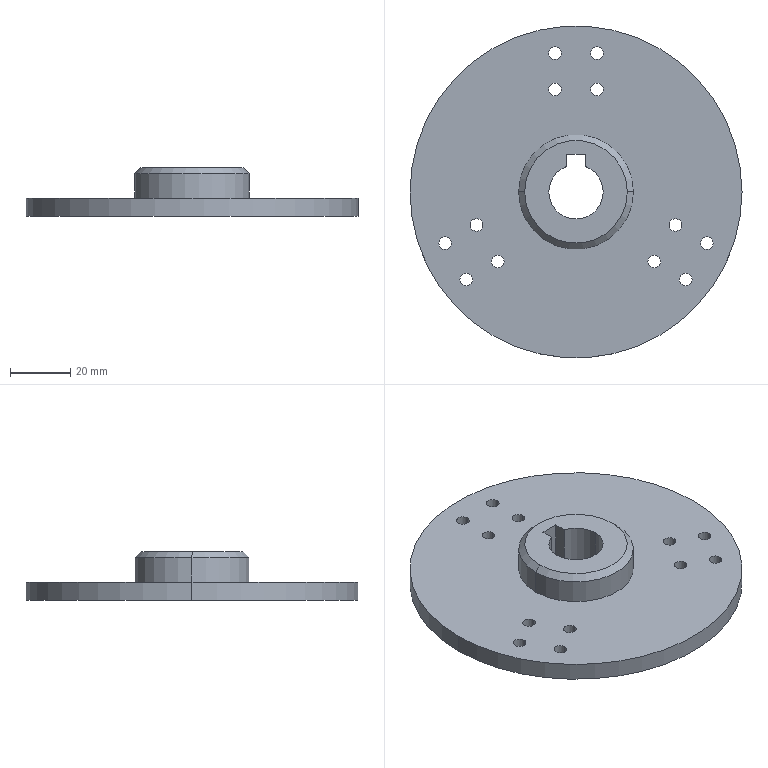Part | STEP file | Cut-off cutter head | 1 solid | 39 faces | box 110 x 110 x 16 mm | volume 62709 mm3 | cylinder 31 | plane 6 | cone 2 | commonest cylinder face diameters 4.2 x24 18 x3 38 x2 110 x2
STEP:
#1=CARTESIAN_POINT('',(17.,0.,16.));
#2=VERTEX_POINT('',#1);
#3=CARTESIAN_POINT('',(-17.,0.,16.));
#4=VERTEX_POINT('',#3);
#5=CARTESIAN_POINT('',(0.,0.,16.));
#6=DIRECTION('',(0.,0.,1.));
#7=DIRECTION('',(1.,0.,0.));
#8=AXIS2_PLACEMENT_3D('',#5,#6,#7);
#9=CIRCLE('',#8,17.);
#10=EDGE_CURVE('',#2,#4,#9,.T.);
#11=ORIENTED_EDGE('',*,*,#10,.F.);
#12=CARTESIAN_POINT('',(19.,0.,14.));
#13=VERTEX_POINT('',#12);
#14=CARTESIAN_POINT('',(17.,0.,16.));
#15=DIRECTION('',(0.7071,0.,-0.7071));
#16=VECTOR('',#15,1000.);
#17=LINE('',#14,#16);
#18=EDGE_CURVE('',#2,#13,#17,.T.);
#19=ORIENTED_EDGE('',*,*,#18,.T.);
#20=CARTESIAN_POINT('',(-19.,0.,14.));
#21=VERTEX_POINT('',#20);
#22=CARTESIAN_POINT('',(0.,0.,14.));
#23=DIRECTION('',(0.,0.,-1.));
#24=DIRECTION('',(1.,0.,0.));
#25=AXIS2_PLACEMENT_3D('',#22,#23,#24);
#26=CIRCLE('',#25,19.);
#27=EDGE_CURVE('',#21,#13,#26,.T.);
#28=ORIENTED_EDGE('',*,*,#27,.F.);
#29=CARTESIAN_POINT('',(-17.,0.,16.));
#30=DIRECTION('',(-0.7071,0.,-0.7071));
#31=VECTOR('',#30,1000.);
#32=LINE('',#29,#31);
#33=EDGE_CURVE('',#4,#21,#32,.T.);
#34=ORIENTED_EDGE('',*,*,#33,.F.);
#35=EDGE_LOOP('',(#11,#19,#28,#34));
#36=FACE_OUTER_BOUND('',#35,.T.);
#37=CARTESIAN_POINT('',(0.,0.,16.));
#38=DIRECTION('',(0.,0.,-1.));
#39=DIRECTION('',(-1.,0.,0.));
#40=AXIS2_PLACEMENT_3D('',#37,#38,#39);
#41=CONICAL_SURFACE('',#40,17.,0.7854);
#42=ADVANCED_FACE('',(#36),#41,.T.);
#43=CARTESIAN_POINT('',(41.237,-16.938,0.));
#44=VERTEX_POINT('',#43);
#45=CARTESIAN_POINT('',(45.437,-16.938,0.));
#46=VERTEX_POINT('',#45);
#47=CARTESIAN_POINT('',(43.337,-16.938,0.));
#48=DIRECTION('',(0.,0.,1.));
#49=DIRECTION('',(1.,0.,0.));
#50=AXIS2_PLACEMENT_3D('',#47,#48,#49);
#51=CIRCLE('',#50,2.1);
#52=EDGE_CURVE('',#44,#46,#51,.T.);
#53=ORIENTED_EDGE('',*,*,#52,.F.);
#54=CARTESIAN_POINT('',(41.237,-16.938,6.));
#55=VERTEX_POINT('',#54);
#56=CARTESIAN_POINT('',(41.237,-16.938,6.));
#57=DIRECTION('',(0.,0.,1.));
#58=VECTOR('',#57,1000.);
#59=LINE('',#56,#58);
#60=EDGE_CURVE('',#44,#55,#59,.T.);
#61=ORIENTED_EDGE('',*,*,#60,.T.);
#62=CARTESIAN_POINT('',(45.437,-16.938,6.));
#63=VERTEX_POINT('',#62);
#64=CARTESIAN_POINT('',(43.337,-16.938,6.));
#65=DIRECTION('',(0.,0.,1.));
#66=DIRECTION('',(1.,0.,0.));
#67=AXIS2_PLACEMENT_3D('',#64,#65,#66);
#68=CIRCLE('',#67,2.1);
#69=EDGE_CURVE('',#55,#63,#68,.T.);
#70=ORIENTED_EDGE('',*,*,#69,.T.);
#71=CARTESIAN_POINT('',(45.437,-16.938,6.));
#72=DIRECTION('',(0.,0.,1.));
#73=VECTOR('',#72,1000.);
#74=LINE('',#71,#73);
#75=EDGE_CURVE('',#46,#63,#74,.T.);
#76=ORIENTED_EDGE('',*,*,#75,.F.);
#77=EDGE_LOOP('',(#53,#61,#70,#76));
#78=FACE_OUTER_BOUND('',#77,.T.);
#79=CARTESIAN_POINT('',(43.337,-16.938,6.));
#80=DIRECTION('',(0.,0.,1.));
#81=DIRECTION('',(1.,0.,0.));
#82=AXIS2_PLACEMENT_3D('',#79,#80,#81);
#83=CYLINDRICAL_SURFACE('',#82,2.1);
#84=ADVANCED_FACE('',(#78),#83,.F.);
#85=CARTESIAN_POINT('',(34.237,-29.062,0.));
#86=VERTEX_POINT('',#85);
#87=CARTESIAN_POINT('',(38.437,-29.062,0.));
#88=VERTEX_POINT('',#87);
#89=CARTESIAN_POINT('',(36.337,-29.062,0.));
#90=DIRECTION('',(0.,0.,1.));
#91=DIRECTION('',(1.,0.,0.));
#92=AXIS2_PLACEMENT_3D('',#89,#90,#91);
#93=CIRCLE('',#92,2.1);
#94=EDGE_CURVE('',#86,#88,#93,.T.);
#95=ORIENTED_EDGE('',*,*,#94,.F.);
#96=CARTESIAN_POINT('',(34.237,-29.062,6.));
#97=VERTEX_POINT('',#96);
#98=CARTESIAN_POINT('',(34.237,-29.062,6.));
#99=DIRECTION('',(0.,0.,1.));
#100=VECTOR('',#99,1000.);
#101=LINE('',#98,#100);
#102=EDGE_CURVE('',#86,#97,#101,.T.);
#103=ORIENTED_EDGE('',*,*,#102,.T.);
#104=CARTESIAN_POINT('',(38.437,-29.062,6.));
#105=VERTEX_POINT('',#104);
#106=CARTESIAN_POINT('',(36.337,-29.062,6.));
#107=DIRECTION('',(0.,0.,1.));
#108=DIRECTION('',(1.,0.,0.));
#109=AXIS2_PLACEMENT_3D('',#106,#107,#108);
#110=CIRCLE('',#109,2.1);
#111=EDGE_CURVE('',#97,#105,#110,.T.);
#112=ORIENTED_EDGE('',*,*,#111,.T.);
#113=CARTESIAN_POINT('',(38.437,-29.062,6.));
#114=DIRECTION('',(0.,0.,1.));
#115=VECTOR('',#114,1000.);
#116=LINE('',#113,#115);
#117=EDGE_CURVE('',#88,#105,#116,.T.);
#118=ORIENTED_EDGE('',*,*,#117,.F.);
#119=EDGE_LOOP('',(#95,#103,#112,#118));
#120=FACE_OUTER_BOUND('',#119,.T.);
#121=CARTESIAN_POINT('',(36.337,-29.062,6.));
#122=DIRECTION('',(0.,0.,1.));
#123=DIRECTION('',(1.,0.,0.));
#124=AXIS2_PLACEMENT_3D('',#121,#122,#123);
#125=CYLINDRICAL_SURFACE('',#124,2.1);
#126=ADVANCED_FACE('',(#120),#125,.F.);
#127=CARTESIAN_POINT('',(23.845,-23.062,0.));
#128=VERTEX_POINT('',#127);
#129=CARTESIAN_POINT('',(28.045,-23.062,0.));
#130=VERTEX_POINT('',#129);
#131=CARTESIAN_POINT('',(25.945,-23.062,0.));
#132=DIRECTION('',(0.,0.,1.));
#133=DIRECTION('',(1.,0.,0.));
#134=AXIS2_PLACEMENT_3D('',#131,#132,#133);
#135=CIRCLE('',#134,2.1);
#136=EDGE_CURVE('',#128,#130,#135,.T.);
#137=ORIENTED_EDGE('',*,*,#136,.F.);
#138=CARTESIAN_POINT('',(23.845,-23.062,6.));
#139=VERTEX_POINT('',#138);
#140=CARTESIAN_POINT('',(23.845,-23.062,6.));
#141=DIRECTION('',(0.,0.,1.));
#142=VECTOR('',#141,1000.);
#143=LINE('',#140,#142);
#144=EDGE_CURVE('',#128,#139,#143,.T.);
#145=ORIENTED_EDGE('',*,*,#144,.T.);
#146=CARTESIAN_POINT('',(28.045,-23.062,6.));
#147=VERTEX_POINT('',#146);
#148=CARTESIAN_POINT('',(25.945,-23.062,6.));
#149=DIRECTION('',(0.,0.,1.));
#150=DIRECTION('',(1.,0.,0.));
#151=AXIS2_PLACEMENT_3D('',#148,#149,#150);
#152=CIRCLE('',#151,2.1);
#153=EDGE_CURVE('',#139,#147,#152,.T.);
#154=ORIENTED_EDGE('',*,*,#153,.T.);
#155=CARTESIAN_POINT('',(28.045,-23.062,6.));
#156=DIRECTION('',(0.,0.,1.));
#157=VECTOR('',#156,1000.);
#158=LINE('',#155,#157);
#159=EDGE_CURVE('',#130,#147,#158,.T.);
#160=ORIENTED_EDGE('',*,*,#159,.F.);
#161=EDGE_LOOP('',(#137,#145,#154,#160));
#162=FACE_OUTER_BOUND('',#161,.T.);
#163=CARTESIAN_POINT('',(25.945,-23.062,6.));
#164=DIRECTION('',(0.,0.,1.));
#165=DIRECTION('',(1.,0.,0.));
#166=AXIS2_PLACEMENT_3D('',#163,#164,#165);
#167=CYLINDRICAL_SURFACE('',#166,2.1);
#168=ADVANCED_FACE('',(#162),#167,.F.);
#169=CARTESIAN_POINT('',(30.845,-10.938,0.));
#170=VERTEX_POINT('',#169);
#171=CARTESIAN_POINT('',(35.045,-10.938,0.));
#172=VERTEX_POINT('',#171);
#173=CARTESIAN_POINT('',(32.945,-10.938,0.));
#174=DIRECTION('',(0.,0.,1.));
#175=DIRECTION('',(1.,0.,0.));
#176=AXIS2_PLACEMENT_3D('',#173,#174,#175);
#177=CIRCLE('',#176,2.1);
#178=EDGE_CURVE('',#170,#172,#177,.T.);
#179=ORIENTED_EDGE('',*,*,#178,.F.);
#180=CARTESIAN_POINT('',(30.845,-10.938,6.));
#181=VERTEX_POINT('',#180);
#182=CARTESIAN_POINT('',(30.845,-10.938,6.));
#183=DIRECTION('',(0.,0.,1.));
#184=VECTOR('',#183,1000.);
#185=LINE('',#182,#184);
#186=EDGE_CURVE('',#170,#181,#185,.T.);
#187=ORIENTED_EDGE('',*,*,#186,.T.);
#188=CARTESIAN_POINT('',(35.045,-10.938,6.));
#189=VERTEX_POINT('',#188);
#190=CARTESIAN_POINT('',(32.945,-10.938,6.));
#191=DIRECTION('',(0.,0.,1.));
#192=DIRECTION('',(1.,0.,0.));
#193=AXIS2_PLACEMENT_3D('',#190,#191,#192);
#194=CIRCLE('',#193,2.1);
#195=EDGE_CURVE('',#181,#189,#194,.T.);
#196=ORIENTED_EDGE('',*,*,#195,.T.);
#197=CARTESIAN_POINT('',(35.045,-10.938,6.));
#198=DIRECTION('',(0.,0.,1.));
#199=VECTOR('',#198,1000.);
#200=LINE('',#197,#199);
#201=EDGE_CURVE('',#172,#189,#200,.T.);
#202=ORIENTED_EDGE('',*,*,#201,.F.);
#203=EDGE_LOOP('',(#179,#187,#196,#202));
#204=FACE_OUTER_BOUND('',#203,.T.);
#205=CARTESIAN_POINT('',(32.945,-10.938,6.));
#206=DIRECTION('',(0.,0.,1.));
#207=DIRECTION('',(1.,0.,0.));
#208=AXIS2_PLACEMENT_3D('',#205,#206,#207);
#209=CYLINDRICAL_SURFACE('',#208,2.1);
#210=ADVANCED_FACE('',(#204),#209,.F.);
#211=CARTESIAN_POINT('',(-38.437,-29.062,0.));
#212=VERTEX_POINT('',#211);
#213=CARTESIAN_POINT('',(-34.237,-29.062,0.));
#214=VERTEX_POINT('',#213);
#215=CARTESIAN_POINT('',(-36.337,-29.062,0.));
#216=DIRECTION('',(0.,0.,1.));
#217=DIRECTION('',(1.,0.,0.));
#218=AXIS2_PLACEMENT_3D('',#215,#216,#217);
#219=CIRCLE('',#218,2.1);
#220=EDGE_CURVE('',#212,#214,#219,.T.);
#221=ORIENTED_EDGE('',*,*,#220,.F.);
#222=CARTESIAN_POINT('',(-38.437,-29.062,6.));
#223=VERTEX_POINT('',#222);
#224=CARTESIAN_POINT('',(-38.437,-29.062,6.));
#225=DIRECTION('',(0.,0.,1.));
#226=VECTOR('',#225,1000.);
#227=LINE('',#224,#226);
#228=EDGE_CURVE('',#212,#223,#227,.T.);
#229=ORIENTED_EDGE('',*,*,#228,.T.);
#230=CARTESIAN_POINT('',(-34.237,-29.062,6.));
#231=VERTEX_POINT('',#230);
#232=CARTESIAN_POINT('',(-36.337,-29.062,6.));
#233=DIRECTION('',(0.,0.,1.));
#234=DIRECTION('',(1.,0.,0.));
#235=AXIS2_PLACEMENT_3D('',#232,#233,#234);
#236=CIRCLE('',#235,2.1);
#237=EDGE_CURVE('',#223,#231,#236,.T.);
#238=ORIENTED_EDGE('',*,*,#237,.T.);
#239=CARTESIAN_POINT('',(-34.237,-29.062,6.));
#240=DIRECTION('',(0.,0.,1.));
#241=VECTOR('',#240,1000.);
#242=LINE('',#239,#241);
#243=EDGE_CURVE('',#214,#231,#242,.T.);
#244=ORIENTED_EDGE('',*,*,#243,.F.);
#245=EDGE_LOOP('',(#221,#229,#238,#244));
#246=FACE_OUTER_BOUND('',#245,.T.);
#247=CARTESIAN_POINT('',(-36.337,-29.062,6.));
#248=DIRECTION('',(0.,0.,1.));
#249=DIRECTION('',(1.,0.,0.));
#250=AXIS2_PLACEMENT_3D('',#247,#248,#249);
#251=CYLINDRICAL_SURFACE('',#250,2.1);
#252=ADVANCED_FACE('',(#246),#251,.F.);
#253=CARTESIAN_POINT('',(-45.437,-16.938,0.));
#254=VERTEX_POINT('',#253);
#255=CARTESIAN_POINT('',(-41.237,-16.938,0.));
#256=VERTEX_POINT('',#255);
#257=CARTESIAN_POINT('',(-43.337,-16.938,0.));
#258=DIRECTION('',(0.,0.,1.));
#259=DIRECTION('',(1.,0.,0.));
#260=AXIS2_PLACEMENT_3D('',#257,#258,#259);
#261=CIRCLE('',#260,2.1);
#262=EDGE_CURVE('',#254,#256,#261,.T.);
#263=ORIENTED_EDGE('',*,*,#262,.F.);
#264=CARTESIAN_POINT('',(-45.437,-16.938,6.));
#265=VERTEX_POINT('',#264);
#266=CARTESIAN_POINT('',(-45.437,-16.938,6.));
#267=DIRECTION('',(0.,0.,1.));
#268=VECTOR('',#267,1000.);
#269=LINE('',#266,#268);
#270=EDGE_CURVE('',#254,#265,#269,.T.);
#271=ORIENTED_EDGE('',*,*,#270,.T.);
#272=CARTESIAN_POINT('',(-41.237,-16.938,6.));
#273=VERTEX_POINT('',#272);
#274=CARTESIAN_POINT('',(-43.337,-16.938,6.));
#275=DIRECTION('',(0.,0.,1.));
#276=DIRECTION('',(1.,0.,0.));
#277=AXIS2_PLACEMENT_3D('',#274,#275,#276);
#278=CIRCLE('',#277,2.1);
#279=EDGE_CURVE('',#265,#273,#278,.T.);
#280=ORIENTED_EDGE('',*,*,#279,.T.);
#281=CARTESIAN_POINT('',(-41.237,-16.938,6.));
#282=DIRECTION('',(0.,0.,1.));
#283=VECTOR('',#282,1000.);
#284=LINE('',#281,#283);
#285=EDGE_CURVE('',#256,#273,#284,.T.);
#286=ORIENTED_EDGE('',*,*,#285,.F.);
#287=EDGE_LOOP('',(#263,#271,#280,#286));
#288=FACE_OUTER_BOUND('',#287,.T.);
#289=CARTESIAN_POINT('',(-43.337,-16.938,6.));
#290=DIRECTION('',(0.,0.,1.));
#291=DIRECTION('',(1.,0.,0.));
#292=AXIS2_PLACEMENT_3D('',#289,#290,#291);
#293=CYLINDRICAL_SURFACE('',#292,2.1);
#294=ADVANCED_FACE('',(#288),#293,.F.);
#295=CARTESIAN_POINT('',(-35.045,-10.938,0.));
#296=VERTEX_POINT('',#295);
#297=CARTESIAN_POINT('',(-30.845,-10.938,0.));
#298=VERTEX_POINT('',#297);
#299=CARTESIAN_POINT('',(-32.945,-10.938,0.));
#300=DIRECTION('',(0.,0.,1.));
#301=DIRECTION('',(1.,0.,0.));
#302=AXIS2_PLACEMENT_3D('',#299,#300,#301);
#303=CIRCLE('',#302,2.1);
#304=EDGE_CURVE('',#296,#298,#303,.T.);
#305=ORIENTED_EDGE('',*,*,#304,.F.);
#306=CARTESIAN_POINT('',(-35.045,-10.938,6.));
#307=VERTEX_POINT('',#306);
#308=CARTESIAN_POINT('',(-35.045,-10.938,6.));
#309=DIRECTION('',(0.,0.,1.));
#310=VECTOR('',#309,1000.);
#311=LINE('',#308,#310);
#312=EDGE_CURVE('',#296,#307,#311,.T.);
#313=ORIENTED_EDGE('',*,*,#312,.T.);
#314=CARTESIAN_POINT('',(-30.845,-10.938,6.));
#315=VERTEX_POINT('',#314);
#316=CARTESIAN_POINT('',(-32.945,-10.938,6.));
#317=DIRECTION('',(0.,0.,1.));
#318=DIRECTION('',(1.,0.,0.));
#319=AXIS2_PLACEMENT_3D('',#316,#317,#318);
#320=CIRCLE('',#319,2.1);
#321=EDGE_CURVE('',#307,#315,#320,.T.);
#322=ORIENTED_EDGE('',*,*,#321,.T.);
#323=CARTESIAN_POINT('',(-30.845,-10.938,6.));
#324=DIRECTION('',(0.,0.,1.));
#325=VECTOR('',#324,1000.);
#326=LINE('',#323,#325);
#327=EDGE_CURVE('',#298,#315,#326,.T.);
#328=ORIENTED_EDGE('',*,*,#327,.F.);
#329=EDGE_LOOP('',(#305,#313,#322,#328));
#330=FACE_OUTER_BOUND('',#329,.T.);
#331=CARTESIAN_POINT('',(-32.945,-10.938,6.));
#332=DIRECTION('',(0.,0.,1.));
#333=DIRECTION('',(1.,0.,0.));
#334=AXIS2_PLACEMENT_3D('',#331,#332,#333);
#335=CYLINDRICAL_SURFACE('',#334,2.1);
#336=ADVANCED_FACE('',(#330),#335,.F.);
#337=CARTESIAN_POINT('',(-28.045,-23.062,0.));
#338=VERTEX_POINT('',#337);
#339=CARTESIAN_POINT('',(-23.845,-23.062,0.));
#340=VERTEX_POINT('',#339);
#341=CARTESIAN_POINT('',(-25.945,-23.062,0.));
#342=DIRECTION('',(0.,0.,1.));
#343=DIRECTION('',(1.,0.,0.));
#344=AXIS2_PLACEMENT_3D('',#341,#342,#343);
#345=CIRCLE('',#344,2.1);
#346=EDGE_CURVE('',#338,#340,#345,.T.);
#347=ORIENTED_EDGE('',*,*,#346,.F.);
#348=CARTESIAN_POINT('',(-28.045,-23.062,6.));
#349=VERTEX_POINT('',#348);
#350=CARTESIAN_POINT('',(-28.045,-23.062,6.));
#351=DIRECTION('',(0.,0.,1.));
#352=VECTOR('',#351,1000.);
#353=LINE('',#350,#352);
#354=EDGE_CURVE('',#338,#349,#353,.T.);
#355=ORIENTED_EDGE('',*,*,#354,.T.);
#356=CARTESIAN_POINT('',(-23.845,-23.062,6.));
#357=VERTEX_POINT('',#356);
#358=CARTESIAN_POINT('',(-25.945,-23.062,6.));
#359=DIRECTION('',(0.,0.,1.));
#360=DIRECTION('',(1.,0.,0.));
#361=AXIS2_PLACEMENT_3D('',#358,#359,#360);
#362=CIRCLE('',#361,2.1);
#363=EDGE_CURVE('',#349,#357,#362,.T.);
#364=ORIENTED_EDGE('',*,*,#363,.T.);
#365=CARTESIAN_POINT('',(-23.845,-23.062,6.));
#366=DIRECTION('',(0.,0.,1.));
#367=VECTOR('',#366,1000.);
#368=LINE('',#365,#367);
#369=EDGE_CURVE('',#340,#357,#368,.T.);
#370=ORIENTED_EDGE('',*,*,#369,.F.);
#371=EDGE_LOOP('',(#347,#355,#364,#370));
#372=FACE_OUTER_BOUND('',#371,.T.);
#373=CARTESIAN_POINT('',(-25.945,-23.062,6.));
#374=DIRECTION('',(0.,0.,1.));
#375=DIRECTION('',(1.,0.,0.));
#376=AXIS2_PLACEMENT_3D('',#373,#374,#375);
#377=CYLINDRICAL_SURFACE('',#376,2.1);
#378=ADVANCED_FACE('',(#372),#377,.F.);
#379=CARTESIAN_POINT('',(-9.1,46.,0.));
#380=VERTEX_POINT('',#379);
#381=CARTESIAN_POINT('',(-4.9,46.,0.));
#382=VERTEX_POINT('',#381);
#383=CARTESIAN_POINT('',(-7.,46.,0.));
#384=DIRECTION('',(0.,0.,1.));
#385=DIRECTION('',(1.,0.,0.));
#386=AXIS2_PLACEMENT_3D('',#383,#384,#385);
#387=CIRCLE('',#386,2.1);
#388=EDGE_CURVE('',#380,#382,#387,.T.);
#389=ORIENTED_EDGE('',*,*,#388,.F.);
#390=CARTESIAN_POINT('',(-9.1,46.,6.));
#391=VERTEX_POINT('',#390);
#392=CARTESIAN_POINT('',(-9.1,46.,6.));
#393=DIRECTION('',(0.,0.,1.));
#394=VECTOR('',#393,1000.);
#395=LINE('',#392,#394);
#396=EDGE_CURVE('',#380,#391,#395,.T.);
#397=ORIENTED_EDGE('',*,*,#396,.T.);
#398=CARTESIAN_POINT('',(-4.9,46.,6.));
#399=VERTEX_POINT('',#398);
#400=CARTESIAN_POINT('',(-7.,46.,6.));
#401=DIRECTION('',(0.,0.,1.));
#402=DIRECTION('',(1.,0.,0.));
#403=AXIS2_PLACEMENT_3D('',#400,#401,#402);
#404=CIRCLE('',#403,2.1);
#405=EDGE_CURVE('',#391,#399,#404,.T.);
#406=ORIENTED_EDGE('',*,*,#405,.T.);
#407=CARTESIAN_POINT('',(-4.9,46.,6.));
#408=DIRECTION('',(0.,0.,1.));
#409=VECTOR('',#408,1000.);
#410=LINE('',#407,#409);
#411=EDGE_CURVE('',#382,#399,#410,.T.);
#412=ORIENTED_EDGE('',*,*,#411,.F.);
#413=EDGE_LOOP('',(#389,#397,#406,#412));
#414=FACE_OUTER_BOUND('',#413,.T.);
#415=CARTESIAN_POINT('',(-7.,46.,6.));
#416=DIRECTION('',(0.,0.,1.));
#417=DIRECTION('',(1.,0.,0.));
#418=AXIS2_PLACEMENT_3D('',#415,#416,#417);
#419=CYLINDRICAL_SURFACE('',#418,2.1);
#420=ADVANCED_FACE('',(#414),#419,.F.);
#421=CARTESIAN_POINT('',(4.9,46.,0.));
#422=VERTEX_POINT('',#421);
#423=CARTESIAN_POINT('',(9.1,46.,0.));
#424=VERTEX_POINT('',#423);
#425=CARTESIAN_POINT('',(7.,46.,0.));
#426=DIRECTION('',(0.,0.,1.));
#427=DIRECTION('',(1.,0.,0.));
#428=AXIS2_PLACEMENT_3D('',#425,#426,#427);
#429=CIRCLE('',#428,2.1);
#430=EDGE_CURVE('',#422,#424,#429,.T.);
#431=ORIENTED_EDGE('',*,*,#430,.F.);
#432=CARTESIAN_POINT('',(4.9,46.,6.));
#433=VERTEX_POINT('',#432);
#434=CARTESIAN_POINT('',(4.9,46.,6.));
#435=DIRECTION('',(0.,0.,1.));
#436=VECTOR('',#435,1000.);
#437=LINE('',#434,#436);
#438=EDGE_CURVE('',#422,#433,#437,.T.);
#439=ORIENTED_EDGE('',*,*,#438,.T.);
#440=CARTESIAN_POINT('',(9.1,46.,6.));
#441=VERTEX_POINT('',#440);
#442=CARTESIAN_POINT('',(7.,46.,6.));
#443=DIRECTION('',(0.,0.,1.));
#444=DIRECTION('',(1.,0.,0.));
#445=AXIS2_PLACEMENT_3D('',#442,#443,#444);
#446=CIRCLE('',#445,2.1);
#447=EDGE_CURVE('',#433,#441,#446,.T.);
#448=ORIENTED_EDGE('',*,*,#447,.T.);
#449=CARTESIAN_POINT('',(9.1,46.,6.));
#450=DIRECTION('',(0.,0.,1.));
#451=VECTOR('',#450,1000.);
#452=LINE('',#449,#451);
#453=EDGE_CURVE('',#424,#441,#452,.T.);
#454=ORIENTED_EDGE('',*,*,#453,.F.);
#455=EDGE_LOOP('',(#431,#439,#448,#454));
#456=FACE_OUTER_BOUND('',#455,.T.);
#457=CARTESIAN_POINT('',(7.,46.,6.));
#458=DIRECTION('',(0.,0.,1.));
#459=DIRECTION('',(1.,0.,0.));
#460=AXIS2_PLACEMENT_3D('',#457,#458,#459);
#461=CYLINDRICAL_SURFACE('',#460,2.1);
#462=ADVANCED_FACE('',(#456),#461,.F.);
#463=CARTESIAN_POINT('',(4.9,34.,0.));
#464=VERTEX_POINT('',#463);
#465=CARTESIAN_POINT('',(9.1,34.,0.));
#466=VERTEX_POINT('',#465);
#467=CARTESIAN_POINT('',(7.,34.,0.));
#468=DIRECTION('',(0.,0.,1.));
#469=DIRECTION('',(1.,0.,0.));
#470=AXIS2_PLACEMENT_3D('',#467,#468,#469);
#471=CIRCLE('',#470,2.1);
#472=EDGE_CURVE('',#464,#466,#471,.T.);
#473=ORIENTED_EDGE('',*,*,#472,.F.);
#474=CARTESIAN_POINT('',(4.9,34.,6.));
#475=VERTEX_POINT('',#474);
#476=CARTESIAN_POINT('',(4.9,34.,6.));
#477=DIRECTION('',(0.,0.,1.));
#478=VECTOR('',#477,1000.);
#479=LINE('',#476,#478);
#480=EDGE_CURVE('',#464,#475,#479,.T.);
#481=ORIENTED_EDGE('',*,*,#480,.T.);
#482=CARTESIAN_POINT('',(9.1,34.,6.));
#483=VERTEX_POINT('',#482);
#484=CARTESIAN_POINT('',(7.,34.,6.));
#485=DIRECTION('',(0.,0.,1.));
#486=DIRECTION('',(1.,0.,0.));
#487=AXIS2_PLACEMENT_3D('',#484,#485,#486);
#488=CIRCLE('',#487,2.1);
#489=EDGE_CURVE('',#475,#483,#488,.T.);
#490=ORIENTED_EDGE('',*,*,#489,.T.);
#491=CARTESIAN_POINT('',(9.1,34.,6.));
#492=DIRECTION('',(0.,0.,1.));
#493=VECTOR('',#492,1000.);
#494=LINE('',#491,#493);
#495=EDGE_CURVE('',#466,#483,#494,.T.);
#496=ORIENTED_EDGE('',*,*,#495,.F.);
#497=EDGE_LOOP('',(#473,#481,#490,#496));
#498=FACE_OUTER_BOUND('',#497,.T.);
#499=CARTESIAN_POINT('',(7.,34.,6.));
#500=DIRECTION('',(0.,0.,1.));
#501=DIRECTION('',(1.,0.,0.));
#502=AXIS2_PLACEMENT_3D('',#499,#500,#501);
#503=CYLINDRICAL_SURFACE('',#502,2.1);
#504=ADVANCED_FACE('',(#498),#503,.F.);
#505=CARTESIAN_POINT('',(-9.1,34.,0.));
#506=VERTEX_POINT('',#505);
#507=CARTESIAN_POINT('',(-4.9,34.,0.));
#508=VERTEX_POINT('',#507);
#509=CARTESIAN_POINT('',(-7.,34.,0.));
#510=DIRECTION('',(0.,0.,1.));
#511=DIRECTION('',(1.,0.,0.));
#512=AXIS2_PLACEMENT_3D('',#509,#510,#511);
#513=CIRCLE('',#512,2.1);
#514=EDGE_CURVE('',#506,#508,#513,.T.);
#515=ORIENTED_EDGE('',*,*,#514,.F.);
#516=CARTESIAN_POINT('',(-9.1,34.,6.));
#517=VERTEX_POINT('',#516);
#518=CARTESIAN_POINT('',(-9.1,34.,6.));
#519=DIRECTION('',(0.,0.,1.));
#520=VECTOR('',#519,1000.);
#521=LINE('',#518,#520);
#522=EDGE_CURVE('',#506,#517,#521,.T.);
#523=ORIENTED_EDGE('',*,*,#522,.T.);
#524=CARTESIAN_POINT('',(-4.9,34.,6.));
#525=VERTEX_POINT('',#524);
#526=CARTESIAN_POINT('',(-7.,34.,6.));
#527=DIRECTION('',(0.,0.,1.));
#528=DIRECTION('',(1.,0.,0.));
#529=AXIS2_PLACEMENT_3D('',#526,#527,#528);
#530=CIRCLE('',#529,2.1);
#531=EDGE_CURVE('',#517,#525,#530,.T.);
#532=ORIENTED_EDGE('',*,*,#531,.T.);
#533=CARTESIAN_POINT('',(-4.9,34.,6.));
#534=DIRECTION('',(0.,0.,1.));
#535=VECTOR('',#534,1000.);
#536=LINE('',#533,#535);
#537=EDGE_CURVE('',#508,#525,#536,.T.);
#538=ORIENTED_EDGE('',*,*,#537,.F.);
#539=EDGE_LOOP('',(#515,#523,#532,#538));
#540=FACE_OUTER_BOUND('',#539,.T.);
#541=CARTESIAN_POINT('',(-7.,34.,6.));
#542=DIRECTION('',(0.,0.,1.));
#543=DIRECTION('',(1.,0.,0.));
#544=AXIS2_PLACEMENT_3D('',#541,#542,#543);
#545=CYLINDRICAL_SURFACE('',#544,2.1);
#546=ADVANCED_FACE('',(#540),#545,.F.);
#547=CARTESIAN_POINT('',(-9.,0.,16.));
#548=VERTEX_POINT('',#547);
#549=CARTESIAN_POINT('',(9.,0.,16.));
#550=VERTEX_POINT('',#549);
#551=CARTESIAN_POINT('',(0.,0.,16.));
#552=DIRECTION('',(0.,0.,1.));
#553=DIRECTION('',(1.,0.,0.));
#554=AXIS2_PLACEMENT_3D('',#551,#552,#553);
#555=CIRCLE('',#554,9.);
#556=EDGE_CURVE('',#548,#550,#555,.T.);
#557=ORIENTED_EDGE('',*,*,#556,.T.);
#558=CARTESIAN_POINT('',(9.,0.,0.));
#559=VERTEX_POINT('',#558);
#560=CARTESIAN_POINT('',(9.,0.,16.));
#561=DIRECTION('',(0.,0.,-1.));
#562=VECTOR('',#561,1000.);
#563=LINE('',#560,#562);
#564=EDGE_CURVE('',#550,#559,#563,.T.);
#565=ORIENTED_EDGE('',*,*,#564,.T.);
#566=CARTESIAN_POINT('',(-9.,0.,0.));
#567=VERTEX_POINT('',#566);
#568=CARTESIAN_POINT('',(0.,0.,0.));
#569=DIRECTION('',(0.,0.,1.));
#570=DIRECTION('',(1.,0.,0.));
#571=AXIS2_PLACEMENT_3D('',#568,#569,#570);
#572=CIRCLE('',#571,9.);
#573=EDGE_CURVE('',#567,#559,#572,.T.);
#574=ORIENTED_EDGE('',*,*,#573,.F.);
#575=CARTESIAN_POINT('',(-9.,0.,16.));
#576=DIRECTION('',(0.,0.,-1.));
#577=VECTOR('',#576,1000.);
#578=LINE('',#575,#577);
#579=EDGE_CURVE('',#548,#567,#578,.T.);
#580=ORIENTED_EDGE('',*,*,#579,.F.);
#581=EDGE_LOOP('',(#557,#565,#574,#580));
#582=FACE_OUTER_BOUND('',#581,.T.);
#583=CARTESIAN_POINT('',(0.,0.,16.));
#584=DIRECTION('',(0.,0.,-1.));
#585=DIRECTION('',(-1.,0.,0.));
#586=AXIS2_PLACEMENT_3D('',#583,#584,#585);
#587=CYLINDRICAL_SURFACE('',#586,9.);
#588=ADVANCED_FACE('',(#582),#587,.F.);
#589=CARTESIAN_POINT('',(-3.,8.485,16.));
#590=VERTEX_POINT('',#589);
#591=CARTESIAN_POINT('',(0.,0.,16.));
#592=DIRECTION('',(0.,0.,1.));
#593=DIRECTION('',(1.,0.,0.));
#594=AXIS2_PLACEMENT_3D('',#591,#592,#593);
#595=CIRCLE('',#594,9.);
#596=EDGE_CURVE('',#590,#548,#595,.T.);
#597=ORIENTED_EDGE('',*,*,#596,.T.);
#598=ORIENTED_EDGE('',*,*,#579,.T.);
#599=CARTESIAN_POINT('',(-3.,8.485,0.));
#600=VERTEX_POINT('',#599);
#601=CARTESIAN_POINT('',(0.,0.,0.));
#602=DIRECTION('',(0.,0.,1.));
#603=DIRECTION('',(1.,0.,0.));
#604=AXIS2_PLACEMENT_3D('',#601,#602,#603);
#605=CIRCLE('',#604,9.);
#606=EDGE_CURVE('',#600,#567,#605,.T.);
#607=ORIENTED_EDGE('',*,*,#606,.F.);
#608=CARTESIAN_POINT('',(-3.,8.485,16.));
#609=DIRECTION('',(0.,0.,-1.));
#610=VECTOR('',#609,1000.);
#611=LINE('',#608,#610);
#612=EDGE_CURVE('',#590,#600,#611,.T.);
#613=ORIENTED_EDGE('',*,*,#612,.F.);
#614=EDGE_LOOP('',(#597,#598,#607,#613));
#615=FACE_OUTER_BOUND('',#614,.T.);
#616=CARTESIAN_POINT('',(0.,0.,16.));
#617=DIRECTION('',(0.,0.,-1.));
#618=DIRECTION('',(-1.,0.,0.));
#619=AXIS2_PLACEMENT_3D('',#616,#617,#618);
#620=CYLINDRICAL_SURFACE('',#619,9.);
#621=ADVANCED_FACE('',(#615),#620,.F.);
#622=ORIENTED_EDGE('',*,*,#27,.T.);
#623=CARTESIAN_POINT('',(19.,0.,6.));
#624=VERTEX_POINT('',#623);
#625=CARTESIAN_POINT('',(19.,0.,16.));
#626=DIRECTION('',(0.,0.,-1.));
#627=VECTOR('',#626,1000.);
#628=LINE('',#625,#627);
#629=EDGE_CURVE('',#13,#624,#628,.T.);
#630=ORIENTED_EDGE('',*,*,#629,.T.);
#631=CARTESIAN_POINT('',(-19.,0.,6.));
#632=VERTEX_POINT('',#631);
#633=CARTESIAN_POINT('',(0.,0.,6.));
#634=DIRECTION('',(0.,0.,1.));
#635=DIRECTION('',(1.,0.,0.));
#636=AXIS2_PLACEMENT_3D('',#633,#634,#635);
#637=CIRCLE('',#636,19.);
#638=EDGE_CURVE('',#624,#632,#637,.T.);
#639=ORIENTED_EDGE('',*,*,#638,.T.);
#640=CARTESIAN_POINT('',(-19.,0.,16.));
#641=DIRECTION('',(0.,0.,-1.));
#642=VECTOR('',#641,1000.);
#643=LINE('',#640,#642);
#644=EDGE_CURVE('',#21,#632,#643,.T.);
#645=ORIENTED_EDGE('',*,*,#644,.F.);
#646=EDGE_LOOP('',(#622,#630,#639,#645));
#647=FACE_OUTER_BOUND('',#646,.T.);
#648=CARTESIAN_POINT('',(0.,0.,16.));
#649=DIRECTION('',(0.,0.,-1.));
#650=DIRECTION('',(-1.,0.,0.));
#651=AXIS2_PLACEMENT_3D('',#648,#649,#650);
#652=CYLINDRICAL_SURFACE('',#651,19.);
#653=ADVANCED_FACE('',(#647),#652,.T.);
#654=CARTESIAN_POINT('',(55.,0.,6.));
#655=VERTEX_POINT('',#654);
#656=CARTESIAN_POINT('',(-55.,0.,6.));
#657=VERTEX_POINT('',#656);
#658=CARTESIAN_POINT('',(0.,0.,6.));
#659=DIRECTION('',(0.,0.,1.));
#660=DIRECTION('',(1.,0.,0.));
#661=AXIS2_PLACEMENT_3D('',#658,#659,#660);
#662=CIRCLE('',#661,55.);
#663=EDGE_CURVE('',#655,#657,#662,.T.);
#664=ORIENTED_EDGE('',*,*,#663,.F.);
#665=CARTESIAN_POINT('',(55.,0.,0.));
#666=VERTEX_POINT('',#665);
#667=CARTESIAN_POINT('',(55.,0.,6.));
#668=DIRECTION('',(0.,0.,-1.));
#669=VECTOR('',#668,1000.);
#670=LINE('',#667,#669);
#671=EDGE_CURVE('',#655,#666,#670,.T.);
#672=ORIENTED_EDGE('',*,*,#671,.T.);
#673=CARTESIAN_POINT('',(-55.,0.,0.));
#674=VERTEX_POINT('',#673);
#675=CARTESIAN_POINT('',(0.,0.,0.));
#676=DIRECTION('',(0.,0.,1.));
#677=DIRECTION('',(1.,0.,0.));
#678=AXIS2_PLACEMENT_3D('',#675,#676,#677);
#679=CIRCLE('',#678,55.);
#680=EDGE_CURVE('',#666,#674,#679,.T.);
#681=ORIENTED_EDGE('',*,*,#680,.T.);
#682=CARTESIAN_POINT('',(-55.,0.,6.));
#683=DIRECTION('',(0.,0.,-1.));
#684=VECTOR('',#683,1000.);
#685=LINE('',#682,#684);
#686=EDGE_CURVE('',#657,#674,#685,.T.);
#687=ORIENTED_EDGE('',*,*,#686,.F.);
#688=EDGE_LOOP('',(#664,#672,#681,#687));
#689=FACE_OUTER_BOUND('',#688,.T.);
#690=CARTESIAN_POINT('',(0.,0.,6.));
#691=DIRECTION('',(0.,0.,-1.));
#692=DIRECTION('',(-1.,0.,0.));
#693=AXIS2_PLACEMENT_3D('',#690,#691,#692);
#694=CYLINDRICAL_SURFACE('',#693,55.);
#695=ADVANCED_FACE('',(#689),#694,.T.);
#696=ORIENTED_EDGE('',*,*,#671,.F.);
#697=CARTESIAN_POINT('',(0.,0.,6.));
#698=DIRECTION('',(0.,0.,1.));
#699=DIRECTION('',(1.,0.,0.));
#700=AXIS2_PLACEMENT_3D('',#697,#698,#699);
#701=CIRCLE('',#700,55.);
#702=EDGE_CURVE('',#657,#655,#701,.T.);
#703=ORIENTED_EDGE('',*,*,#702,.F.);
#704=ORIENTED_EDGE('',*,*,#686,.T.);
#705=CARTESIAN_POINT('',(0.,0.,0.));
#706=DIRECTION('',(0.,0.,1.));
#707=DIRECTION('',(1.,0.,0.));
#708=AXIS2_PLACEMENT_3D('',#705,#706,#707);
#709=CIRCLE('',#708,55.);
#710=EDGE_CURVE('',#674,#666,#709,.T.);
#711=ORIENTED_EDGE('',*,*,#710,.T.);
#712=EDGE_LOOP('',(#696,#703,#704,#711));
#713=FACE_OUTER_BOUND('',#712,.T.);
#714=CARTESIAN_POINT('',(0.,0.,6.));
#715=DIRECTION('',(0.,0.,-1.));
#716=DIRECTION('',(-1.,0.,0.));
#717=AXIS2_PLACEMENT_3D('',#714,#715,#716);
#718=CYLINDRICAL_SURFACE('',#717,55.);
#719=ADVANCED_FACE('',(#713),#718,.T.);
#720=CARTESIAN_POINT('',(43.337,-16.938,6.));
#721=DIRECTION('',(0.,0.,1.));
#722=DIRECTION('',(1.,0.,0.));
#723=AXIS2_PLACEMENT_3D('',#720,#721,#722);
#724=CIRCLE('',#723,2.1);
#725=EDGE_CURVE('',#63,#55,#724,.T.);
#726=ORIENTED_EDGE('',*,*,#725,.F.);
#727=ORIENTED_EDGE('',*,*,#69,.F.);
#728=EDGE_LOOP('',(#726,#727));
#729=FACE_BOUND('',#728,.T.);
#730=CARTESIAN_POINT('',(36.337,-29.062,6.));
#731=DIRECTION('',(0.,0.,1.));
#732=DIRECTION('',(1.,0.,0.));
#733=AXIS2_PLACEMENT_3D('',#730,#731,#732);
#734=CIRCLE('',#733,2.1);
#735=EDGE_CURVE('',#105,#97,#734,.T.);
#736=ORIENTED_EDGE('',*,*,#735,.F.);
#737=ORIENTED_EDGE('',*,*,#111,.F.);
#738=EDGE_LOOP('',(#736,#737));
#739=FACE_BOUND('',#738,.T.);
#740=CARTESIAN_POINT('',(25.945,-23.062,6.));
#741=DIRECTION('',(0.,0.,1.));
#742=DIRECTION('',(1.,0.,0.));
#743=AXIS2_PLACEMENT_3D('',#740,#741,#742);
#744=CIRCLE('',#743,2.1);
#745=EDGE_CURVE('',#147,#139,#744,.T.);
#746=ORIENTED_EDGE('',*,*,#745,.F.);
#747=ORIENTED_EDGE('',*,*,#153,.F.);
#748=EDGE_LOOP('',(#746,#747));
#749=FACE_BOUND('',#748,.T.);
#750=CARTESIAN_POINT('',(32.945,-10.938,6.));
#751=DIRECTION('',(0.,0.,1.));
#752=DIRECTION('',(1.,0.,0.));
#753=AXIS2_PLACEMENT_3D('',#750,#751,#752);
#754=CIRCLE('',#753,2.1);
#755=EDGE_CURVE('',#189,#181,#754,.T.);
#756=ORIENTED_EDGE('',*,*,#755,.F.);
#757=ORIENTED_EDGE('',*,*,#195,.F.);
#758=EDGE_LOOP('',(#756,#757));
#759=FACE_BOUND('',#758,.T.);
#760=CARTESIAN_POINT('',(-36.337,-29.062,6.));
#761=DIRECTION('',(0.,0.,1.));
#762=DIRECTION('',(1.,0.,0.));
#763=AXIS2_PLACEMENT_3D('',#760,#761,#762);
#764=CIRCLE('',#763,2.1);
#765=EDGE_CURVE('',#231,#223,#764,.T.);
#766=ORIENTED_EDGE('',*,*,#765,.F.);
#767=ORIENTED_EDGE('',*,*,#237,.F.);
#768=EDGE_LOOP('',(#766,#767));
#769=FACE_BOUND('',#768,.T.);
#770=CARTESIAN_POINT('',(-43.337,-16.938,6.));
#771=DIRECTION('',(0.,0.,1.));
#772=DIRECTION('',(1.,0.,0.));
#773=AXIS2_PLACEMENT_3D('',#770,#771,#772);
#774=CIRCLE('',#773,2.1);
#775=EDGE_CURVE('',#273,#265,#774,.T.);
#776=ORIENTED_EDGE('',*,*,#775,.F.);
#777=ORIENTED_EDGE('',*,*,#279,.F.);
#778=EDGE_LOOP('',(#776,#777));
#779=FACE_BOUND('',#778,.T.);
#780=CARTESIAN_POINT('',(-32.945,-10.938,6.));
#781=DIRECTION('',(0.,0.,1.));
#782=DIRECTION('',(1.,0.,0.));
#783=AXIS2_PLACEMENT_3D('',#780,#781,#782);
#784=CIRCLE('',#783,2.1);
#785=EDGE_CURVE('',#315,#307,#784,.T.);
#786=ORIENTED_EDGE('',*,*,#785,.F.);
#787=ORIENTED_EDGE('',*,*,#321,.F.);
#788=EDGE_LOOP('',(#786,#787));
#789=FACE_BOUND('',#788,.T.);
#790=CARTESIAN_POINT('',(-25.945,-23.062,6.));
#791=DIRECTION('',(0.,0.,1.));
#792=DIRECTION('',(1.,0.,0.));
#793=AXIS2_PLACEMENT_3D('',#790,#791,#792);
#794=CIRCLE('',#793,2.1);
#795=EDGE_CURVE('',#357,#349,#794,.T.);
#796=ORIENTED_EDGE('',*,*,#795,.F.);
#797=ORIENTED_EDGE('',*,*,#363,.F.);
#798=EDGE_LOOP('',(#796,#797));
#799=FACE_BOUND('',#798,.T.);
#800=CARTESIAN_POINT('',(-7.,46.,6.));
#801=DIRECTION('',(0.,0.,1.));
#802=DIRECTION('',(1.,0.,0.));
#803=AXIS2_PLACEMENT_3D('',#800,#801,#802);
#804=CIRCLE('',#803,2.1);
#805=EDGE_CURVE('',#399,#391,#804,.T.);
#806=ORIENTED_EDGE('',*,*,#805,.F.);
#807=ORIENTED_EDGE('',*,*,#405,.F.);
#808=EDGE_LOOP('',(#806,#807));
#809=FACE_BOUND('',#808,.T.);
#810=CARTESIAN_POINT('',(7.,46.,6.));
#811=DIRECTION('',(0.,0.,1.));
#812=DIRECTION('',(1.,0.,0.));
#813=AXIS2_PLACEMENT_3D('',#810,#811,#812);
#814=CIRCLE('',#813,2.1);
#815=EDGE_CURVE('',#441,#433,#814,.T.);
#816=ORIENTED_EDGE('',*,*,#815,.F.);
#817=ORIENTED_EDGE('',*,*,#447,.F.);
#818=EDGE_LOOP('',(#816,#817));
#819=FACE_BOUND('',#818,.T.);
#820=CARTESIAN_POINT('',(7.,34.,6.));
#821=DIRECTION('',(0.,0.,1.));
#822=DIRECTION('',(1.,0.,0.));
#823=AXIS2_PLACEMENT_3D('',#820,#821,#822);
#824=CIRCLE('',#823,2.1);
#825=EDGE_CURVE('',#483,#475,#824,.T.);
#826=ORIENTED_EDGE('',*,*,#825,.F.);
#827=ORIENTED_EDGE('',*,*,#489,.F.);
#828=EDGE_LOOP('',(#826,#827));
#829=FACE_BOUND('',#828,.T.);
#830=CARTESIAN_POINT('',(-7.,34.,6.));
#831=DIRECTION('',(0.,0.,1.));
#832=DIRECTION('',(1.,0.,0.));
#833=AXIS2_PLACEMENT_3D('',#830,#831,#832);
#834=CIRCLE('',#833,2.1);
#835=EDGE_CURVE('',#525,#517,#834,.T.);
#836=ORIENTED_EDGE('',*,*,#835,.F.);
#837=ORIENTED_EDGE('',*,*,#531,.F.);
#838=EDGE_LOOP('',(#836,#837));
#839=FACE_BOUND('',#838,.T.);
#840=CARTESIAN_POINT('',(0.,0.,6.));
#841=DIRECTION('',(0.,0.,1.));
#842=DIRECTION('',(1.,0.,0.));
#843=AXIS2_PLACEMENT_3D('',#840,#841,#842);
#844=CIRCLE('',#843,19.);
#845=EDGE_CURVE('',#632,#624,#844,.T.);
#846=ORIENTED_EDGE('',*,*,#845,.F.);
#847=ORIENTED_EDGE('',*,*,#638,.F.);
#848=EDGE_LOOP('',(#846,#847));
#849=FACE_BOUND('',#848,.T.);
#850=ORIENTED_EDGE('',*,*,#702,.T.);
#851=ORIENTED_EDGE('',*,*,#663,.T.);
#852=EDGE_LOOP('',(#850,#851));
#853=FACE_OUTER_BOUND('',#852,.T.);
#854=CARTESIAN_POINT('',(0.,0.,6.));
#855=DIRECTION('',(0.,0.,1.));
#856=DIRECTION('',(1.,0.,0.));
#857=AXIS2_PLACEMENT_3D('',#854,#855,#856);
#858=PLANE('',#857);
#859=ADVANCED_FACE('',(#729,#739,#749,#759,#769,#779,#789,#799,#809,#819,#829,#839,#849,#853),#858,.T.);
#860=ORIENTED_EDGE('',*,*,#606,.T.);
#861=ORIENTED_EDGE('',*,*,#573,.T.);
#862=CARTESIAN_POINT('',(3.,8.485,0.));
#863=VERTEX_POINT('',#862);
#864=CARTESIAN_POINT('',(0.,0.,0.));
#865=DIRECTION('',(0.,0.,1.));
#866=DIRECTION('',(1.,0.,0.));
#867=AXIS2_PLACEMENT_3D('',#864,#865,#866);
#868=CIRCLE('',#867,9.);
#869=EDGE_CURVE('',#559,#863,#868,.T.);
#870=ORIENTED_EDGE('',*,*,#869,.T.);
#871=CARTESIAN_POINT('',(3.,12.5,0.));
#872=VERTEX_POINT('',#871);
#873=CARTESIAN_POINT('',(3.,0.,0.));
#874=DIRECTION('',(0.,1.,0.));
#875=VECTOR('',#874,1000.);
#876=LINE('',#873,#875);
#877=EDGE_CURVE('',#863,#872,#876,.T.);
#878=ORIENTED_EDGE('',*,*,#877,.T.);
#879=CARTESIAN_POINT('',(-3.,12.5,0.));
#880=VERTEX_POINT('',#879);
#881=CARTESIAN_POINT('',(0.,12.5,0.));
#882=DIRECTION('',(-1.,0.,0.));
#883=VECTOR('',#882,1000.);
#884=LINE('',#881,#883);
#885=EDGE_CURVE('',#872,#880,#884,.T.);
#886=ORIENTED_EDGE('',*,*,#885,.T.);
#887=CARTESIAN_POINT('',(-3.,0.,0.));
#888=DIRECTION('',(0.,-1.,0.));
#889=VECTOR('',#888,1000.);
#890=LINE('',#887,#889);
#891=EDGE_CURVE('',#880,#600,#890,.T.);
#892=ORIENTED_EDGE('',*,*,#891,.T.);
#893=EDGE_LOOP('',(#860,#861,#870,#878,#886,#892));
#894=FACE_BOUND('',#893,.T.);
#895=CARTESIAN_POINT('',(43.337,-16.938,0.));
#896=DIRECTION('',(0.,0.,1.));
#897=DIRECTION('',(1.,0.,0.));
#898=AXIS2_PLACEMENT_3D('',#895,#896,#897);
#899=CIRCLE('',#898,2.1);
#900=EDGE_CURVE('',#46,#44,#899,.T.);
#901=ORIENTED_EDGE('',*,*,#900,.T.);
#902=ORIENTED_EDGE('',*,*,#52,.T.);
#903=EDGE_LOOP('',(#901,#902));
#904=FACE_BOUND('',#903,.T.);
#905=CARTESIAN_POINT('',(36.337,-29.062,0.));
#906=DIRECTION('',(0.,0.,1.));
#907=DIRECTION('',(1.,0.,0.));
#908=AXIS2_PLACEMENT_3D('',#905,#906,#907);
#909=CIRCLE('',#908,2.1);
#910=EDGE_CURVE('',#88,#86,#909,.T.);
#911=ORIENTED_EDGE('',*,*,#910,.T.);
#912=ORIENTED_EDGE('',*,*,#94,.T.);
#913=EDGE_LOOP('',(#911,#912));
#914=FACE_BOUND('',#913,.T.);
#915=CARTESIAN_POINT('',(25.945,-23.062,0.));
#916=DIRECTION('',(0.,0.,1.));
#917=DIRECTION('',(1.,0.,0.));
#918=AXIS2_PLACEMENT_3D('',#915,#916,#917);
#919=CIRCLE('',#918,2.1);
#920=EDGE_CURVE('',#130,#128,#919,.T.);
#921=ORIENTED_EDGE('',*,*,#920,.T.);
#922=ORIENTED_EDGE('',*,*,#136,.T.);
#923=EDGE_LOOP('',(#921,#922));
#924=FACE_BOUND('',#923,.T.);
#925=CARTESIAN_POINT('',(32.945,-10.938,0.));
#926=DIRECTION('',(0.,0.,1.));
#927=DIRECTION('',(1.,0.,0.));
#928=AXIS2_PLACEMENT_3D('',#925,#926,#927);
#929=CIRCLE('',#928,2.1);
#930=EDGE_CURVE('',#172,#170,#929,.T.);
#931=ORIENTED_EDGE('',*,*,#930,.T.);
#932=ORIENTED_EDGE('',*,*,#178,.T.);
#933=EDGE_LOOP('',(#931,#932));
#934=FACE_BOUND('',#933,.T.);
#935=CARTESIAN_POINT('',(-36.337,-29.062,0.));
#936=DIRECTION('',(0.,0.,1.));
#937=DIRECTION('',(1.,0.,0.));
#938=AXIS2_PLACEMENT_3D('',#935,#936,#937);
#939=CIRCLE('',#938,2.1);
#940=EDGE_CURVE('',#214,#212,#939,.T.);
#941=ORIENTED_EDGE('',*,*,#940,.T.);
#942=ORIENTED_EDGE('',*,*,#220,.T.);
#943=EDGE_LOOP('',(#941,#942));
#944=FACE_BOUND('',#943,.T.);
#945=CARTESIAN_POINT('',(-43.337,-16.938,0.));
#946=DIRECTION('',(0.,0.,1.));
#947=DIRECTION('',(1.,0.,0.));
#948=AXIS2_PLACEMENT_3D('',#945,#946,#947);
#949=CIRCLE('',#948,2.1);
#950=EDGE_CURVE('',#256,#254,#949,.T.);
#951=ORIENTED_EDGE('',*,*,#950,.T.);
#952=ORIENTED_EDGE('',*,*,#262,.T.);
#953=EDGE_LOOP('',(#951,#952));
#954=FACE_BOUND('',#953,.T.);
#955=CARTESIAN_POINT('',(-32.945,-10.938,0.));
#956=DIRECTION('',(0.,0.,1.));
#957=DIRECTION('',(1.,0.,0.));
#958=AXIS2_PLACEMENT_3D('',#955,#956,#957);
#959=CIRCLE('',#958,2.1);
#960=EDGE_CURVE('',#298,#296,#959,.T.);
#961=ORIENTED_EDGE('',*,*,#960,.T.);
#962=ORIENTED_EDGE('',*,*,#304,.T.);
#963=EDGE_LOOP('',(#961,#962));
#964=FACE_BOUND('',#963,.T.);
#965=CARTESIAN_POINT('',(-25.945,-23.062,0.));
#966=DIRECTION('',(0.,0.,1.));
#967=DIRECTION('',(1.,0.,0.));
#968=AXIS2_PLACEMENT_3D('',#965,#966,#967);
#969=CIRCLE('',#968,2.1);
#970=EDGE_CURVE('',#340,#338,#969,.T.);
#971=ORIENTED_EDGE('',*,*,#970,.T.);
#972=ORIENTED_EDGE('',*,*,#346,.T.);
#973=EDGE_LOOP('',(#971,#972));
#974=FACE_BOUND('',#973,.T.);
#975=CARTESIAN_POINT('',(-7.,46.,0.));
#976=DIRECTION('',(0.,0.,1.));
#977=DIRECTION('',(1.,0.,0.));
#978=AXIS2_PLACEMENT_3D('',#975,#976,#977);
#979=CIRCLE('',#978,2.1);
#980=EDGE_CURVE('',#382,#380,#979,.T.);
#981=ORIENTED_EDGE('',*,*,#980,.T.);
#982=ORIENTED_EDGE('',*,*,#388,.T.);
#983=EDGE_LOOP('',(#981,#982));
#984=FACE_BOUND('',#983,.T.);
#985=CARTESIAN_POINT('',(7.,46.,0.));
#986=DIRECTION('',(0.,0.,1.));
#987=DIRECTION('',(1.,0.,0.));
#988=AXIS2_PLACEMENT_3D('',#985,#986,#987);
#989=CIRCLE('',#988,2.1);
#990=EDGE_CURVE('',#424,#422,#989,.T.);
#991=ORIENTED_EDGE('',*,*,#990,.T.);
#992=ORIENTED_EDGE('',*,*,#430,.T.);
#993=EDGE_LOOP('',(#991,#992));
#994=FACE_BOUND('',#993,.T.);
#995=CARTESIAN_POINT('',(7.,34.,0.));
#996=DIRECTION('',(0.,0.,1.));
#997=DIRECTION('',(1.,0.,0.));
#998=AXIS2_PLACEMENT_3D('',#995,#996,#997);
#999=CIRCLE('',#998,2.1);
#1000=EDGE_CURVE('',#466,#464,#999,.T.);
#1001=ORIENTED_EDGE('',*,*,#1000,.T.);
#1002=ORIENTED_EDGE('',*,*,#472,.T.);
#1003=EDGE_LOOP('',(#1001,#1002));
#1004=FACE_BOUND('',#1003,.T.);
#1005=CARTESIAN_POINT('',(-7.,34.,0.));
#1006=DIRECTION('',(0.,0.,1.));
#1007=DIRECTION('',(1.,0.,0.));
#1008=AXIS2_PLACEMENT_3D('',#1005,#1006,#1007);
#1009=CIRCLE('',#1008,2.1);
#1010=EDGE_CURVE('',#508,#506,#1009,.T.);
#1011=ORIENTED_EDGE('',*,*,#1010,.T.);
#1012=ORIENTED_EDGE('',*,*,#514,.T.);
#1013=EDGE_LOOP('',(#1011,#1012));
#1014=FACE_BOUND('',#1013,.T.);
#1015=ORIENTED_EDGE('',*,*,#710,.F.);
#1016=ORIENTED_EDGE('',*,*,#680,.F.);
#1017=EDGE_LOOP('',(#1015,#1016));
#1018=FACE_OUTER_BOUND('',#1017,.T.);
#1019=CARTESIAN_POINT('',(0.,0.,0.));
#1020=DIRECTION('',(0.,0.,1.));
#1021=DIRECTION('',(1.,0.,0.));
#1022=AXIS2_PLACEMENT_3D('',#1019,#1020,#1021);
#1023=PLANE('',#1022);
#1024=ADVANCED_FACE('',(#894,#904,#914,#924,#934,#944,#954,#964,#974,#984,#994,#1004,#1014,#1018),#1023,.F.);
#1025=CARTESIAN_POINT('',(0.,0.,16.));
#1026=DIRECTION('',(0.,0.,1.));
#1027=DIRECTION('',(1.,0.,0.));
#1028=AXIS2_PLACEMENT_3D('',#1025,#1026,#1027);
#1029=CIRCLE('',#1028,17.);
#1030=EDGE_CURVE('',#4,#2,#1029,.T.);
#1031=ORIENTED_EDGE('',*,*,#1030,.T.);
#1032=ORIENTED_EDGE('',*,*,#10,.T.);
#1033=EDGE_LOOP('',(#1031,#1032));
#1034=FACE_OUTER_BOUND('',#1033,.T.);
#1035=CARTESIAN_POINT('',(3.,8.485,16.));
#1036=VERTEX_POINT('',#1035);
#1037=CARTESIAN_POINT('',(3.,12.5,16.));
#1038=VERTEX_POINT('',#1037);
#1039=CARTESIAN_POINT('',(3.,12.5,16.));
#1040=DIRECTION('',(0.,1.,0.));
#1041=VECTOR('',#1040,1000.);
#1042=LINE('',#1039,#1041);
#1043=EDGE_CURVE('',#1036,#1038,#1042,.T.);
#1044=ORIENTED_EDGE('',*,*,#1043,.F.);
#1045=CARTESIAN_POINT('',(0.,0.,16.));
#1046=DIRECTION('',(0.,0.,1.));
#1047=DIRECTION('',(1.,0.,0.));
#1048=AXIS2_PLACEMENT_3D('',#1045,#1046,#1047);
#1049=CIRCLE('',#1048,9.);
#1050=EDGE_CURVE('',#550,#1036,#1049,.T.);
#1051=ORIENTED_EDGE('',*,*,#1050,.F.);
#1052=ORIENTED_EDGE('',*,*,#556,.F.);
#1053=ORIENTED_EDGE('',*,*,#596,.F.);
#1054=CARTESIAN_POINT('',(-3.,12.5,16.));
#1055=VERTEX_POINT('',#1054);
#1056=CARTESIAN_POINT('',(-3.,12.5,16.));
#1057=DIRECTION('',(0.,-1.,0.));
#1058=VECTOR('',#1057,1000.);
#1059=LINE('',#1056,#1058);
#1060=EDGE_CURVE('',#1055,#590,#1059,.T.);
#1061=ORIENTED_EDGE('',*,*,#1060,.F.);
#1062=CARTESIAN_POINT('',(-3.,12.5,16.));
#1063=DIRECTION('',(-1.,0.,0.));
#1064=VECTOR('',#1063,1000.);
#1065=LINE('',#1062,#1064);
#1066=EDGE_CURVE('',#1038,#1055,#1065,.T.);
#1067=ORIENTED_EDGE('',*,*,#1066,.F.);
#1068=EDGE_LOOP('',(#1044,#1051,#1052,#1053,#1061,#1067));
#1069=FACE_BOUND('',#1068,.T.);
#1070=CARTESIAN_POINT('',(0.,0.,16.));
#1071=DIRECTION('',(0.,0.,1.));
#1072=DIRECTION('',(1.,0.,0.));
#1073=AXIS2_PLACEMENT_3D('',#1070,#1071,#1072);
#1074=PLANE('',#1073);
#1075=ADVANCED_FACE('',(#1034,#1069),#1074,.T.);
#1076=ORIENTED_EDGE('',*,*,#629,.F.);
#1077=CARTESIAN_POINT('',(0.,0.,14.));
#1078=DIRECTION('',(0.,0.,-1.));
#1079=DIRECTION('',(1.,0.,0.));
#1080=AXIS2_PLACEMENT_3D('',#1077,#1078,#1079);
#1081=CIRCLE('',#1080,19.);
#1082=EDGE_CURVE('',#13,#21,#1081,.T.);
#1083=ORIENTED_EDGE('',*,*,#1082,.T.);
#1084=ORIENTED_EDGE('',*,*,#644,.T.);
#1085=ORIENTED_EDGE('',*,*,#845,.T.);
#1086=EDGE_LOOP('',(#1076,#1083,#1084,#1085));
#1087=FACE_OUTER_BOUND('',#1086,.T.);
#1088=CARTESIAN_POINT('',(0.,0.,16.));
#1089=DIRECTION('',(0.,0.,-1.));
#1090=DIRECTION('',(-1.,0.,0.));
#1091=AXIS2_PLACEMENT_3D('',#1088,#1089,#1090);
#1092=CYLINDRICAL_SURFACE('',#1091,19.);
#1093=ADVANCED_FACE('',(#1087),#1092,.T.);
#1094=ORIENTED_EDGE('',*,*,#564,.F.);
#1095=ORIENTED_EDGE('',*,*,#1050,.T.);
#1096=CARTESIAN_POINT('',(3.,8.485,16.));
#1097=DIRECTION('',(0.,0.,1.));
#1098=VECTOR('',#1097,1000.);
#1099=LINE('',#1096,#1098);
#1100=EDGE_CURVE('',#863,#1036,#1099,.T.);
#1101=ORIENTED_EDGE('',*,*,#1100,.F.);
#1102=ORIENTED_EDGE('',*,*,#869,.F.);
#1103=EDGE_LOOP('',(#1094,#1095,#1101,#1102));
#1104=FACE_OUTER_BOUND('',#1103,.T.);
#1105=CARTESIAN_POINT('',(0.,0.,16.));
#1106=DIRECTION('',(0.,0.,-1.));
#1107=DIRECTION('',(-1.,0.,0.));
#1108=AXIS2_PLACEMENT_3D('',#1105,#1106,#1107);
#1109=CYLINDRICAL_SURFACE('',#1108,9.);
#1110=ADVANCED_FACE('',(#1104),#1109,.F.);
#1111=ORIENTED_EDGE('',*,*,#522,.F.);
#1112=ORIENTED_EDGE('',*,*,#1010,.F.);
#1113=ORIENTED_EDGE('',*,*,#537,.T.);
#1114=ORIENTED_EDGE('',*,*,#835,.T.);
#1115=EDGE_LOOP('',(#1111,#1112,#1113,#1114));
#1116=FACE_OUTER_BOUND('',#1115,.T.);
#1117=CARTESIAN_POINT('',(-7.,34.,6.));
#1118=DIRECTION('',(0.,0.,1.));
#1119=DIRECTION('',(1.,0.,0.));
#1120=AXIS2_PLACEMENT_3D('',#1117,#1118,#1119);
#1121=CYLINDRICAL_SURFACE('',#1120,2.1);
#1122=ADVANCED_FACE('',(#1116),#1121,.F.);
#1123=ORIENTED_EDGE('',*,*,#480,.F.);
#1124=ORIENTED_EDGE('',*,*,#1000,.F.);
#1125=ORIENTED_EDGE('',*,*,#495,.T.);
#1126=ORIENTED_EDGE('',*,*,#825,.T.);
#1127=EDGE_LOOP('',(#1123,#1124,#1125,#1126));
#1128=FACE_OUTER_BOUND('',#1127,.T.);
#1129=CARTESIAN_POINT('',(7.,34.,6.));
#1130=DIRECTION('',(0.,0.,1.));
#1131=DIRECTION('',(1.,0.,0.));
#1132=AXIS2_PLACEMENT_3D('',#1129,#1130,#1131);
#1133=CYLINDRICAL_SURFACE('',#1132,2.1);
#1134=ADVANCED_FACE('',(#1128),#1133,.F.);
#1135=ORIENTED_EDGE('',*,*,#438,.F.);
#1136=ORIENTED_EDGE('',*,*,#990,.F.);
#1137=ORIENTED_EDGE('',*,*,#453,.T.);
#1138=ORIENTED_EDGE('',*,*,#815,.T.);
#1139=EDGE_LOOP('',(#1135,#1136,#1137,#1138));
#1140=FACE_OUTER_BOUND('',#1139,.T.);
#1141=CARTESIAN_POINT('',(7.,46.,6.));
#1142=DIRECTION('',(0.,0.,1.));
#1143=DIRECTION('',(1.,0.,0.));
#1144=AXIS2_PLACEMENT_3D('',#1141,#1142,#1143);
#1145=CYLINDRICAL_SURFACE('',#1144,2.1);
#1146=ADVANCED_FACE('',(#1140),#1145,.F.);
#1147=ORIENTED_EDGE('',*,*,#396,.F.);
#1148=ORIENTED_EDGE('',*,*,#980,.F.);
#1149=ORIENTED_EDGE('',*,*,#411,.T.);
#1150=ORIENTED_EDGE('',*,*,#805,.T.);
#1151=EDGE_LOOP('',(#1147,#1148,#1149,#1150));
#1152=FACE_OUTER_BOUND('',#1151,.T.);
#1153=CARTESIAN_POINT('',(-7.,46.,6.));
#1154=DIRECTION('',(0.,0.,1.));
#1155=DIRECTION('',(1.,0.,0.));
#1156=AXIS2_PLACEMENT_3D('',#1153,#1154,#1155);
#1157=CYLINDRICAL_SURFACE('',#1156,2.1);
#1158=ADVANCED_FACE('',(#1152),#1157,.F.);
#1159=ORIENTED_EDGE('',*,*,#354,.F.);
#1160=ORIENTED_EDGE('',*,*,#970,.F.);
#1161=ORIENTED_EDGE('',*,*,#369,.T.);
#1162=ORIENTED_EDGE('',*,*,#795,.T.);
#1163=EDGE_LOOP('',(#1159,#1160,#1161,#1162));
#1164=FACE_OUTER_BOUND('',#1163,.T.);
#1165=CARTESIAN_POINT('',(-25.945,-23.062,6.));
#1166=DIRECTION('',(0.,0.,1.));
#1167=DIRECTION('',(1.,0.,0.));
#1168=AXIS2_PLACEMENT_3D('',#1165,#1166,#1167);
#1169=CYLINDRICAL_SURFACE('',#1168,2.1);
#1170=ADVANCED_FACE('',(#1164),#1169,.F.);
#1171=ORIENTED_EDGE('',*,*,#312,.F.);
#1172=ORIENTED_EDGE('',*,*,#960,.F.);
#1173=ORIENTED_EDGE('',*,*,#327,.T.);
#1174=ORIENTED_EDGE('',*,*,#785,.T.);
#1175=EDGE_LOOP('',(#1171,#1172,#1173,#1174));
#1176=FACE_OUTER_BOUND('',#1175,.T.);
#1177=CARTESIAN_POINT('',(-32.945,-10.938,6.));
#1178=DIRECTION('',(0.,0.,1.));
#1179=DIRECTION('',(1.,0.,0.));
#1180=AXIS2_PLACEMENT_3D('',#1177,#1178,#1179);
#1181=CYLINDRICAL_SURFACE('',#1180,2.1);
#1182=ADVANCED_FACE('',(#1176),#1181,.F.);
#1183=ORIENTED_EDGE('',*,*,#270,.F.);
#1184=ORIENTED_EDGE('',*,*,#950,.F.);
#1185=ORIENTED_EDGE('',*,*,#285,.T.);
#1186=ORIENTED_EDGE('',*,*,#775,.T.);
#1187=EDGE_LOOP('',(#1183,#1184,#1185,#1186));
#1188=FACE_OUTER_BOUND('',#1187,.T.);
#1189=CARTESIAN_POINT('',(-43.337,-16.938,6.));
#1190=DIRECTION('',(0.,0.,1.));
#1191=DIRECTION('',(1.,0.,0.));
#1192=AXIS2_PLACEMENT_3D('',#1189,#1190,#1191);
#1193=CYLINDRICAL_SURFACE('',#1192,2.1);
#1194=ADVANCED_FACE('',(#1188),#1193,.F.);
#1195=ORIENTED_EDGE('',*,*,#228,.F.);
#1196=ORIENTED_EDGE('',*,*,#940,.F.);
#1197=ORIENTED_EDGE('',*,*,#243,.T.);
#1198=ORIENTED_EDGE('',*,*,#765,.T.);
#1199=EDGE_LOOP('',(#1195,#1196,#1197,#1198));
#1200=FACE_OUTER_BOUND('',#1199,.T.);
#1201=CARTESIAN_POINT('',(-36.337,-29.062,6.));
#1202=DIRECTION('',(0.,0.,1.));
#1203=DIRECTION('',(1.,0.,0.));
#1204=AXIS2_PLACEMENT_3D('',#1201,#1202,#1203);
#1205=CYLINDRICAL_SURFACE('',#1204,2.1);
#1206=ADVANCED_FACE('',(#1200),#1205,.F.);
#1207=ORIENTED_EDGE('',*,*,#186,.F.);
#1208=ORIENTED_EDGE('',*,*,#930,.F.);
#1209=ORIENTED_EDGE('',*,*,#201,.T.);
#1210=ORIENTED_EDGE('',*,*,#755,.T.);
#1211=EDGE_LOOP('',(#1207,#1208,#1209,#1210));
#1212=FACE_OUTER_BOUND('',#1211,.T.);
#1213=CARTESIAN_POINT('',(32.945,-10.938,6.));
#1214=DIRECTION('',(0.,0.,1.));
#1215=DIRECTION('',(1.,0.,0.));
#1216=AXIS2_PLACEMENT_3D('',#1213,#1214,#1215);
#1217=CYLINDRICAL_SURFACE('',#1216,2.1);
#1218=ADVANCED_FACE('',(#1212),#1217,.F.);
#1219=ORIENTED_EDGE('',*,*,#144,.F.);
#1220=ORIENTED_EDGE('',*,*,#920,.F.);
#1221=ORIENTED_EDGE('',*,*,#159,.T.);
#1222=ORIENTED_EDGE('',*,*,#745,.T.);
#1223=EDGE_LOOP('',(#1219,#1220,#1221,#1222));
#1224=FACE_OUTER_BOUND('',#1223,.T.);
#1225=CARTESIAN_POINT('',(25.945,-23.062,6.));
#1226=DIRECTION('',(0.,0.,1.));
#1227=DIRECTION('',(1.,0.,0.));
#1228=AXIS2_PLACEMENT_3D('',#1225,#1226,#1227);
#1229=CYLINDRICAL_SURFACE('',#1228,2.1);
#1230=ADVANCED_FACE('',(#1224),#1229,.F.);
#1231=ORIENTED_EDGE('',*,*,#102,.F.);
#1232=ORIENTED_EDGE('',*,*,#910,.F.);
#1233=ORIENTED_EDGE('',*,*,#117,.T.);
#1234=ORIENTED_EDGE('',*,*,#735,.T.);
#1235=EDGE_LOOP('',(#1231,#1232,#1233,#1234));
#1236=FACE_OUTER_BOUND('',#1235,.T.);
#1237=CARTESIAN_POINT('',(36.337,-29.062,6.));
#1238=DIRECTION('',(0.,0.,1.));
#1239=DIRECTION('',(1.,0.,0.));
#1240=AXIS2_PLACEMENT_3D('',#1237,#1238,#1239);
#1241=CYLINDRICAL_SURFACE('',#1240,2.1);
#1242=ADVANCED_FACE('',(#1236),#1241,.F.);
#1243=ORIENTED_EDGE('',*,*,#60,.F.);
#1244=ORIENTED_EDGE('',*,*,#900,.F.);
#1245=ORIENTED_EDGE('',*,*,#75,.T.);
#1246=ORIENTED_EDGE('',*,*,#725,.T.);
#1247=EDGE_LOOP('',(#1243,#1244,#1245,#1246));
#1248=FACE_OUTER_BOUND('',#1247,.T.);
#1249=CARTESIAN_POINT('',(43.337,-16.938,6.));
#1250=DIRECTION('',(0.,0.,1.));
#1251=DIRECTION('',(1.,0.,0.));
#1252=AXIS2_PLACEMENT_3D('',#1249,#1250,#1251);
#1253=CYLINDRICAL_SURFACE('',#1252,2.1);
#1254=ADVANCED_FACE('',(#1248),#1253,.F.);
#1255=CARTESIAN_POINT('',(3.,12.5,-10.));
#1256=DIRECTION('',(0.,0.,1.));
#1257=VECTOR('',#1256,1000.);
#1258=LINE('',#1255,#1257);
#1259=EDGE_CURVE('',#872,#1038,#1258,.T.);
#1260=ORIENTED_EDGE('',*,*,#1259,.T.);
#1261=ORIENTED_EDGE('',*,*,#1066,.T.);
#1262=CARTESIAN_POINT('',(-3.,12.5,-10.));
#1263=DIRECTION('',(0.,0.,1.));
#1264=VECTOR('',#1263,1000.);
#1265=LINE('',#1262,#1264);
#1266=EDGE_CURVE('',#880,#1055,#1265,.T.);
#1267=ORIENTED_EDGE('',*,*,#1266,.F.);
#1268=ORIENTED_EDGE('',*,*,#885,.F.);
#1269=EDGE_LOOP('',(#1260,#1261,#1267,#1268));
#1270=FACE_OUTER_BOUND('',#1269,.T.);
#1271=CARTESIAN_POINT('',(-3.,12.5,-10.));
#1272=DIRECTION('',(0.,1.,0.));
#1273=DIRECTION('',(0.,0.,1.));
#1274=AXIS2_PLACEMENT_3D('',#1271,#1272,#1273);
#1275=PLANE('',#1274);
#1276=ADVANCED_FACE('',(#1270),#1275,.F.);
#1277=ORIENTED_EDGE('',*,*,#1100,.T.);
#1278=ORIENTED_EDGE('',*,*,#1043,.T.);
#1279=ORIENTED_EDGE('',*,*,#1259,.F.);
#1280=ORIENTED_EDGE('',*,*,#877,.F.);
#1281=EDGE_LOOP('',(#1277,#1278,#1279,#1280));
#1282=FACE_OUTER_BOUND('',#1281,.T.);
#1283=CARTESIAN_POINT('',(3.,12.5,-10.));
#1284=DIRECTION('',(1.,0.,0.));
#1285=DIRECTION('',(0.,1.,0.));
#1286=AXIS2_PLACEMENT_3D('',#1283,#1284,#1285);
#1287=PLANE('',#1286);
#1288=ADVANCED_FACE('',(#1282),#1287,.F.);
#1289=ORIENTED_EDGE('',*,*,#1266,.T.);
#1290=ORIENTED_EDGE('',*,*,#1060,.T.);
#1291=ORIENTED_EDGE('',*,*,#612,.T.);
#1292=ORIENTED_EDGE('',*,*,#891,.F.);
#1293=EDGE_LOOP('',(#1289,#1290,#1291,#1292));
#1294=FACE_OUTER_BOUND('',#1293,.T.);
#1295=CARTESIAN_POINT('',(-3.,12.5,-10.));
#1296=DIRECTION('',(-1.,0.,0.));
#1297=DIRECTION('',(0.,-1.,0.));
#1298=AXIS2_PLACEMENT_3D('',#1295,#1296,#1297);
#1299=PLANE('',#1298);
#1300=ADVANCED_FACE('',(#1294),#1299,.F.);
#1301=ORIENTED_EDGE('',*,*,#18,.F.);
#1302=ORIENTED_EDGE('',*,*,#1030,.F.);
#1303=ORIENTED_EDGE('',*,*,#33,.T.);
#1304=ORIENTED_EDGE('',*,*,#1082,.F.);
#1305=EDGE_LOOP('',(#1301,#1302,#1303,#1304));
#1306=FACE_OUTER_BOUND('',#1305,.T.);
#1307=CARTESIAN_POINT('',(0.,0.,16.));
#1308=DIRECTION('',(0.,0.,-1.));
#1309=DIRECTION('',(-1.,0.,0.));
#1310=AXIS2_PLACEMENT_3D('',#1307,#1308,#1309);
#1311=CONICAL_SURFACE('',#1310,17.,0.7854);
#1312=ADVANCED_FACE('',(#1306),#1311,.T.);
#1313=CLOSED_SHELL('',(#42,#84,#126,#168,#210,#252,#294,#336,#378,#420,#462,#504,#546,#588,#621,#653,#695,#719,#859,#1024,#1075,#1093,#1110,#1122,#1134,#1146,#1158,#1170,#1182,#1194,#1206,#1218,#1230,#1242,#1254,#1276,#1288,#1300,#1312));
#1314=MANIFOLD_SOLID_BREP('',#1313);
#1315=CARTESIAN_POINT('',(0.,0.,0.));
#1316=DIRECTION('',(0.,0.,1.));
#1317=DIRECTION('',(1.,0.,0.));
#1318=AXIS2_PLACEMENT_3D('',#1315,#1316,#1317);
#1319=(LENGTH_UNIT()NAMED_UNIT(*)SI_UNIT(.MILLI.,.METRE.));
#1320=UNCERTAINTY_MEASURE_WITH_UNIT(LENGTH_MEASURE(0.00001),#1319,'','');
#1321=(NAMED_UNIT(*)PLANE_ANGLE_UNIT()SI_UNIT($,.RADIAN.));
#1322=(NAMED_UNIT(*)SI_UNIT($,.STERADIAN.)SOLID_ANGLE_UNIT());
#1323=(GEOMETRIC_REPRESENTATION_CONTEXT(3)GLOBAL_UNCERTAINTY_ASSIGNED_CONTEXT((#1320))GLOBAL_UNIT_ASSIGNED_CONTEXT((#1319,#1321,#1322))REPRESENTATION_CONTEXT('',''));
#1324=ADVANCED_BREP_SHAPE_REPRESENTATION('',(#1314,#1318),#1323);